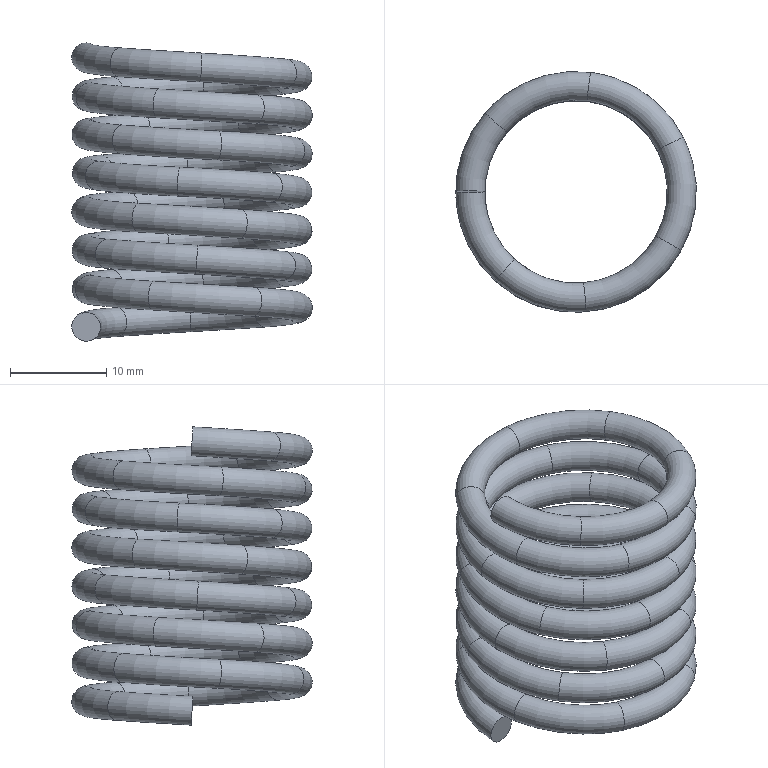Part | NX | features solid 2 | 1 solid | 48 faces | box 25.01 x 25.011 x 30.995 mm | volume 3423 mm3 | torus 46 | plane 2
STEP:
#1=CARTESIAN_POINT('',(-1547.251,422.027,-15.808));
#2=VERTEX_POINT('',#1);
#3=CARTESIAN_POINT('',(-1547.85,422.702,-17.006));
#4=DIRECTION('',(-0.6998,-0.7125,-0.05188));
#5=DIRECTION('',(0.3989,-0.45,0.799));
#6=AXIS2_PLACEMENT_3D('',#3,#4,#5);
#7=CIRCLE('',#6,1.5);
#8=EDGE_CURVE('',#2,#2,#7,.T.);
#9=ORIENTED_EDGE('',*,*,#8,.T.);
#10=EDGE_LOOP('',(#9));
#11=FACE_BOUND('',#10,.T.);
#12=CARTESIAN_POINT('',(-1550.155,414.928,-16.263));
#13=VERTEX_POINT('',#12);
#14=CARTESIAN_POINT('',(-1551.,415.,-17.5));
#15=DIRECTION('',(0.,-0.9983,-0.05778));
#16=DIRECTION('',(0.5635,-0.04773,0.8248));
#17=AXIS2_PLACEMENT_3D('',#14,#15,#16);
#18=CIRCLE('',#17,1.5);
#19=EDGE_CURVE('',#13,#13,#18,.T.);
#20=ORIENTED_EDGE('',*,*,#19,.F.);
#21=EDGE_LOOP('',(#20));
#22=FACE_BOUND('',#21,.T.);
#23=CARTESIAN_POINT('',(-1539.974,414.99,-17.333));
#24=DIRECTION('',(-0.01519,-0.05777,0.9982));
#25=DIRECTION('',(0.,-0.9983,-0.05778));
#26=AXIS2_PLACEMENT_3D('',#23,#24,#25);
#27=TOROIDAL_SURFACE('',#26,11.027,1.5);
#28=ADVANCED_FACE('',(#11,#22),#27,.T.);
#29=CARTESIAN_POINT('',(-1540.254,425.044,-15.355));
#30=VERTEX_POINT('',#29);
#31=CARTESIAN_POINT('',(-1540.206,425.998,-16.512));
#32=DIRECTION('',(-0.9981,-0.01974,-0.05793));
#33=DIRECTION('',(-0.03218,-0.6359,0.7711));
#34=AXIS2_PLACEMENT_3D('',#31,#32,#33);
#35=CIRCLE('',#34,1.5);
#36=EDGE_CURVE('',#30,#30,#35,.T.);
#37=ORIENTED_EDGE('',*,*,#36,.T.);
#38=EDGE_LOOP('',(#37));
#39=FACE_BOUND('',#38,.T.);
#40=ORIENTED_EDGE('',*,*,#8,.F.);
#41=EDGE_LOOP('',(#40));
#42=FACE_BOUND('',#41,.T.);
#43=CARTESIAN_POINT('',(-1539.978,414.946,-16.677));
#44=DIRECTION('',(-0.05762,-0.0161,0.9982));
#45=DIRECTION('',(0.9983,0.,0.05762));
#46=AXIS2_PLACEMENT_3D('',#43,#44,#45);
#47=TOROIDAL_SURFACE('',#46,11.056,1.5);
#48=ADVANCED_FACE('',(#39,#42),#47,.T.);
#49=CARTESIAN_POINT('',(-1533.181,422.306,-14.905));
#50=VERTEX_POINT('',#49);
#51=CARTESIAN_POINT('',(-1532.449,422.995,-16.018));
#52=DIRECTION('',(-0.725,0.6868,-0.05181));
#53=DIRECTION('',(-0.4882,-0.4594,0.742));
#54=AXIS2_PLACEMENT_3D('',#51,#52,#53);
#55=CIRCLE('',#54,1.5);
#56=EDGE_CURVE('',#50,#50,#55,.T.);
#57=ORIENTED_EDGE('',*,*,#56,.T.);
#58=EDGE_LOOP('',(#57));
#59=FACE_BOUND('',#58,.T.);
#60=ORIENTED_EDGE('',*,*,#36,.F.);
#61=EDGE_LOOP('',(#60));
#62=FACE_BOUND('',#61,.T.);
#63=CARTESIAN_POINT('',(-1539.998,415.002,-16.347));
#64=DIRECTION('',(-0.05821,0.01386,0.9982));
#65=DIRECTION('',(0.9983,0.,0.05821));
#66=AXIS2_PLACEMENT_3D('',#63,#64,#65);
#67=TOROIDAL_SURFACE('',#66,11.,1.5);
#68=ADVANCED_FACE('',(#59,#62),#67,.T.);
#69=CARTESIAN_POINT('',(-1530.062,415.432,-14.457));
#70=VERTEX_POINT('',#69);
#71=CARTESIAN_POINT('',(-1529.008,415.412,-15.524));
#72=DIRECTION('',(-0.03934,0.9975,-0.05792));
#73=DIRECTION('',(-0.7028,0.01358,0.7112));
#74=AXIS2_PLACEMENT_3D('',#71,#72,#73);
#75=CIRCLE('',#74,1.5);
#76=EDGE_CURVE('',#70,#70,#75,.T.);
#77=ORIENTED_EDGE('',*,*,#76,.T.);
#78=EDGE_LOOP('',(#77));
#79=FACE_BOUND('',#78,.T.);
#80=ORIENTED_EDGE('',*,*,#56,.F.);
#81=EDGE_LOOP('',(#80));
#82=FACE_BOUND('',#81,.T.);
#83=CARTESIAN_POINT('',(-1540.079,414.966,-15.688));
#84=DIRECTION('',(-0.01706,0.05729,0.9982));
#85=DIRECTION('',(0.,-0.9984,0.0573));
#86=AXIS2_PLACEMENT_3D('',#83,#84,#85);
#87=TOROIDAL_SURFACE('',#86,11.081,1.5);
#88=ADVANCED_FACE('',(#79,#82),#87,.T.);
#89=CARTESIAN_POINT('',(-1534.223,406.975,-13.888));
#90=VERTEX_POINT('',#89);
#91=CARTESIAN_POINT('',(-1533.618,406.04,-14.893));
#92=DIRECTION('',(0.8145,0.5782,-0.04816));
#93=DIRECTION('',(-0.4029,0.6233,0.6702));
#94=AXIS2_PLACEMENT_3D('',#91,#92,#93);
#95=CIRCLE('',#94,1.5);
#96=EDGE_CURVE('',#90,#90,#95,.T.);
#97=ORIENTED_EDGE('',*,*,#96,.T.);
#98=EDGE_LOOP('',(#97));
#99=FACE_BOUND('',#98,.T.);
#100=ORIENTED_EDGE('',*,*,#76,.F.);
#101=EDGE_LOOP('',(#100));
#102=FACE_BOUND('',#101,.T.);
#103=CARTESIAN_POINT('',(-1539.997,414.991,-15.308));
#104=DIRECTION('',(0.01738,0.05864,0.9981));
#105=DIRECTION('',(0.,-0.9983,0.05865));
#106=AXIS2_PLACEMENT_3D('',#103,#104,#105);
#107=TOROIDAL_SURFACE('',#106,10.999,1.5);
#108=ADVANCED_FACE('',(#99,#102),#107,.T.);
#109=CARTESIAN_POINT('',(-1543.516,405.833,-13.323));
#110=VERTEX_POINT('',#109);
#111=CARTESIAN_POINT('',(-1543.992,404.765,-14.263));
#112=DIRECTION('',(0.9297,-0.3638,-0.05774));
#113=DIRECTION('',(0.3175,0.7119,0.6264));
#114=AXIS2_PLACEMENT_3D('',#111,#112,#113);
#115=CIRCLE('',#114,1.5);
#116=EDGE_CURVE('',#110,#110,#115,.T.);
#117=ORIENTED_EDGE('',*,*,#116,.T.);
#118=EDGE_LOOP('',(#117));
#119=FACE_BOUND('',#118,.T.);
#120=ORIENTED_EDGE('',*,*,#96,.F.);
#121=EDGE_LOOP('',(#120));
#122=FACE_BOUND('',#121,.T.);
#123=CARTESIAN_POINT('',(-1539.984,415.041,-14.48));
#124=DIRECTION('',(0.06093,-0.002702,0.9981));
#125=DIRECTION('',(0.9981,0.,-0.06093));
#126=AXIS2_PLACEMENT_3D('',#123,#124,#125);
#127=TOROIDAL_SURFACE('',#126,11.033,1.5);
#128=ADVANCED_FACE('',(#119,#122),#127,.T.);
#129=CARTESIAN_POINT('',(-1549.456,412.582,-12.782));
#130=VERTEX_POINT('',#129);
#131=CARTESIAN_POINT('',(-1550.647,412.328,-13.657));
#132=DIRECTION('',(0.243,-0.9688,-0.04909));
#133=DIRECTION('',(0.7946,0.1697,0.583));
#134=AXIS2_PLACEMENT_3D('',#131,#132,#133);
#135=CIRCLE('',#134,1.5);
#136=EDGE_CURVE('',#130,#130,#135,.T.);
#137=ORIENTED_EDGE('',*,*,#136,.T.);
#138=EDGE_LOOP('',(#137));
#139=FACE_BOUND('',#138,.T.);
#140=ORIENTED_EDGE('',*,*,#116,.F.);
#141=EDGE_LOOP('',(#140));
#142=FACE_BOUND('',#141,.T.);
#143=CARTESIAN_POINT('',(-1539.963,415.027,-14.053));
#144=DIRECTION('',(0.04679,-0.03884,0.9981));
#145=DIRECTION('',(0.9989,0.,-0.04683));
#146=AXIS2_PLACEMENT_3D('',#143,#144,#145);
#147=TOROIDAL_SURFACE('',#146,11.027,1.5);
#148=ADVANCED_FACE('',(#139,#142),#147,.T.);
#149=CARTESIAN_POINT('',(-1547.425,421.291,-12.244));
#150=VERTEX_POINT('',#149);
#151=CARTESIAN_POINT('',(-1548.358,422.145,-13.05));
#152=DIRECTION('',(-0.6463,-0.7609,-0.05788));
#153=DIRECTION('',(0.6222,-0.5694,0.5373));
#154=AXIS2_PLACEMENT_3D('',#151,#152,#153);
#155=CIRCLE('',#154,1.5);
#156=EDGE_CURVE('',#150,#150,#155,.T.);
#157=ORIENTED_EDGE('',*,*,#156,.T.);
#158=EDGE_LOOP('',(#157));
#159=FACE_BOUND('',#158,.T.);
#160=ORIENTED_EDGE('',*,*,#136,.F.);
#161=EDGE_LOOP('',(#160));
#162=FACE_BOUND('',#161,.T.);
#163=CARTESIAN_POINT('',(-1539.924,414.997,-13.259));
#164=DIRECTION('',(-0.02304,-0.05635,0.9981));
#165=DIRECTION('',(0.,-0.9984,-0.05637));
#166=AXIS2_PLACEMENT_3D('',#163,#164,#165);
#167=TOROIDAL_SURFACE('',#166,11.057,1.5);
#168=ADVANCED_FACE('',(#159,#162),#167,.T.);
#169=CARTESIAN_POINT('',(-1538.882,424.631,-11.69));
#170=VERTEX_POINT('',#169);
#171=CARTESIAN_POINT('',(-1538.689,425.925,-12.423));
#172=DIRECTION('',(-0.9915,0.1205,-0.04827));
#173=DIRECTION('',(-0.1286,-0.863,0.4886));
#174=AXIS2_PLACEMENT_3D('',#171,#172,#173);
#175=CIRCLE('',#174,1.5);
#176=EDGE_CURVE('',#170,#170,#175,.T.);
#177=ORIENTED_EDGE('',*,*,#176,.T.);
#178=EDGE_LOOP('',(#177));
#179=FACE_BOUND('',#178,.T.);
#180=ORIENTED_EDGE('',*,*,#156,.F.);
#181=EDGE_LOOP('',(#180));
#182=FACE_BOUND('',#181,.T.);
#183=CARTESIAN_POINT('',(-1539.994,415.023,-12.835));
#184=DIRECTION('',(-0.0524,-0.03142,0.9981));
#185=DIRECTION('',(0.9986,0.,0.05243));
#186=AXIS2_PLACEMENT_3D('',#183,#184,#185);
#187=TOROIDAL_SURFACE('',#186,10.987,1.5);
#188=ADVANCED_FACE('',(#179,#182),#187,.T.);
#189=CARTESIAN_POINT('',(-1531.412,419.377,-11.14));
#190=VERTEX_POINT('',#189);
#191=CARTESIAN_POINT('',(-1530.191,419.947,-11.797));
#192=DIRECTION('',(-0.448,0.8921,-0.05774));
#193=DIRECTION('',(-0.8144,-0.3806,0.4381));
#194=AXIS2_PLACEMENT_3D('',#191,#192,#193);
#195=CIRCLE('',#194,1.5);
#196=EDGE_CURVE('',#190,#190,#195,.T.);
#197=ORIENTED_EDGE('',*,*,#196,.T.);
#198=EDGE_LOOP('',(#197));
#199=FACE_BOUND('',#198,.T.);
#200=ORIENTED_EDGE('',*,*,#176,.F.);
#201=EDGE_LOOP('',(#200));
#202=FACE_BOUND('',#201,.T.);
#203=CARTESIAN_POINT('',(-1540.038,414.988,-12.013));
#204=DIRECTION('',(-0.04338,0.04282,0.9981));
#205=DIRECTION('',(0.9991,0.,0.04342));
#206=AXIS2_PLACEMENT_3D('',#203,#204,#205);
#207=TOROIDAL_SURFACE('',#206,11.028,1.5);
#208=ADVANCED_FACE('',(#199,#202),#207,.T.);
#209=CARTESIAN_POINT('',(-1531.72,410.149,-10.583));
#210=VERTEX_POINT('',#209);
#211=CARTESIAN_POINT('',(-1530.541,409.424,-11.162));
#212=DIRECTION('',(0.5065,0.8609,-0.04814));
#213=DIRECTION('',(-0.7856,0.4837,0.3859));
#214=AXIS2_PLACEMENT_3D('',#211,#212,#213);
#215=CIRCLE('',#214,1.5);
#216=EDGE_CURVE('',#210,#210,#215,.T.);
#217=ORIENTED_EDGE('',*,*,#216,.T.);
#218=EDGE_LOOP('',(#217));
#219=FACE_BOUND('',#218,.T.);
#220=ORIENTED_EDGE('',*,*,#196,.F.);
#221=EDGE_LOOP('',(#220));
#222=FACE_BOUND('',#221,.T.);
#223=CARTESIAN_POINT('',(-1540.065,415.003,-11.577));
#224=DIRECTION('',(-0.00806,0.06056,0.9981));
#225=DIRECTION('',(0.,-0.9982,0.06056));
#226=AXIS2_PLACEMENT_3D('',#223,#224,#225);
#227=TOROIDAL_SURFACE('',#226,11.045,1.5);
#228=ADVANCED_FACE('',(#219,#222),#227,.T.);
#229=CARTESIAN_POINT('',(-1539.599,405.424,-10.027));
#230=VERTEX_POINT('',#229);
#231=CARTESIAN_POINT('',(-1539.569,404.009,-10.525));
#232=DIRECTION('',(0.9975,0.04112,-0.05792));
#233=DIRECTION('',(-0.0196,0.9431,0.3319));
#234=AXIS2_PLACEMENT_3D('',#231,#232,#233);
#235=CIRCLE('',#234,1.5);
#236=EDGE_CURVE('',#230,#230,#235,.T.);
#237=ORIENTED_EDGE('',*,*,#236,.T.);
#238=EDGE_LOOP('',(#237));
#239=FACE_BOUND('',#238,.T.);
#240=ORIENTED_EDGE('',*,*,#216,.F.);
#241=EDGE_LOOP('',(#240));
#242=FACE_BOUND('',#241,.T.);
#243=CARTESIAN_POINT('',(-1540.036,415.033,-10.744));
#244=DIRECTION('',(0.05704,0.02226,0.9981));
#245=DIRECTION('',(0.9984,0.,-0.05706));
#246=AXIS2_PLACEMENT_3D('',#243,#244,#245);
#247=TOROIDAL_SURFACE('',#246,11.036,1.5);
#248=ADVANCED_FACE('',(#239,#242),#247,.T.);
#249=CARTESIAN_POINT('',(-1547.65,409.26,-9.49));
#250=VERTEX_POINT('',#249);
#251=CARTESIAN_POINT('',(-1548.817,408.415,-9.908));
#252=DIRECTION('',(0.597,-0.8008,-0.04853));
#253=DIRECTION('',(0.778,0.5631,0.2787));
#254=AXIS2_PLACEMENT_3D('',#251,#252,#253);
#255=CIRCLE('',#254,1.5);
#256=EDGE_CURVE('',#250,#250,#255,.T.);
#257=ORIENTED_EDGE('',*,*,#256,.T.);
#258=EDGE_LOOP('',(#257));
#259=FACE_BOUND('',#258,.T.);
#260=ORIENTED_EDGE('',*,*,#236,.F.);
#261=EDGE_LOOP('',(#260));
#262=FACE_BOUND('',#261,.T.);
#263=CARTESIAN_POINT('',(-1540.01,415.005,-10.314));
#264=DIRECTION('',(0.05865,-0.01676,0.9981));
#265=DIRECTION('',(0.9983,0.,-0.05866));
#266=AXIS2_PLACEMENT_3D('',#263,#264,#265);
#267=TOROIDAL_SURFACE('',#266,11.007,1.5);
#268=ADVANCED_FACE('',(#259,#262),#267,.T.);
#269=CARTESIAN_POINT('',(-1549.026,418.045,-8.955));
#270=VERTEX_POINT('',#269);
#271=CARTESIAN_POINT('',(-1550.402,418.537,-9.291));
#272=DIRECTION('',(-0.3236,-0.9444,-0.05775));
#273=DIRECTION('',(0.9176,-0.3282,0.2244));
#274=AXIS2_PLACEMENT_3D('',#271,#272,#273);
#275=CIRCLE('',#274,1.5);
#276=EDGE_CURVE('',#270,#270,#275,.T.);
#277=ORIENTED_EDGE('',*,*,#276,.T.);
#278=EDGE_LOOP('',(#277));
#279=FACE_BOUND('',#278,.T.);
#280=ORIENTED_EDGE('',*,*,#256,.F.);
#281=EDGE_LOOP('',(#280));
#282=FACE_BOUND('',#281,.T.);
#283=CARTESIAN_POINT('',(-1539.98,414.978,-9.503));
#284=DIRECTION('',(-0.0005035,-0.06086,0.9981));
#285=DIRECTION('',(0.,-0.9981,-0.06086));
#286=AXIS2_PLACEMENT_3D('',#283,#284,#285);
#287=TOROIDAL_SURFACE('',#286,11.015,1.5);
#288=ADVANCED_FACE('',(#279,#282),#287,.T.);
#289=CARTESIAN_POINT('',(-1542.436,424.179,-8.412));
#290=VERTEX_POINT('',#289);
#291=CARTESIAN_POINT('',(-1542.802,425.612,-8.665));
#292=DIRECTION('',(-0.9655,-0.2557,-0.04849));
#293=DIRECTION('',(0.2444,-0.9549,0.1689));
#294=AXIS2_PLACEMENT_3D('',#291,#292,#293);
#295=CIRCLE('',#294,1.5);
#296=EDGE_CURVE('',#290,#290,#295,.T.);
#297=ORIENTED_EDGE('',*,*,#296,.T.);
#298=EDGE_LOOP('',(#297));
#299=FACE_BOUND('',#298,.T.);
#300=ORIENTED_EDGE('',*,*,#276,.F.);
#301=EDGE_LOOP('',(#300));
#302=FACE_BOUND('',#301,.T.);
#303=CARTESIAN_POINT('',(-1539.957,414.944,-9.074));
#304=DIRECTION('',(-0.03735,-0.04823,0.9981));
#305=DIRECTION('',(0.,-0.9988,-0.04827));
#306=AXIS2_PLACEMENT_3D('',#303,#304,#305);
#307=TOROIDAL_SURFACE('',#306,11.048,1.5);
#308=ADVANCED_FACE('',(#299,#302),#307,.T.);
#309=CARTESIAN_POINT('',(-1533.693,422.112,-7.869));
#310=VERTEX_POINT('',#309);
#311=CARTESIAN_POINT('',(-1532.699,423.223,-8.038));
#312=DIRECTION('',(-0.7482,0.6609,-0.05789));
#313=DIRECTION('',(-0.6627,-0.7404,0.1126));
#314=AXIS2_PLACEMENT_3D('',#311,#312,#313);
#315=CIRCLE('',#314,1.5);
#316=EDGE_CURVE('',#310,#310,#315,.T.);
#317=ORIENTED_EDGE('',*,*,#316,.T.);
#318=EDGE_LOOP('',(#317));
#319=FACE_BOUND('',#318,.T.);
#320=ORIENTED_EDGE('',*,*,#296,.F.);
#321=EDGE_LOOP('',(#320));
#322=FACE_BOUND('',#321,.T.);
#323=CARTESIAN_POINT('',(-1539.997,414.941,-8.254));
#324=DIRECTION('',(-0.05637,0.0236,0.9981));
#325=DIRECTION('',(0.9984,0.,0.05639));
#326=AXIS2_PLACEMENT_3D('',#323,#324,#325);
#327=TOROIDAL_SURFACE('',#326,11.041,1.5);
#328=ADVANCED_FACE('',(#319,#322),#327,.T.);
#329=CARTESIAN_POINT('',(-1530.566,413.83,-7.335));
#330=VERTEX_POINT('',#329);
#331=CARTESIAN_POINT('',(-1529.081,413.639,-7.42));
#332=DIRECTION('',(0.1246,0.991,-0.04854));
#333=DIRECTION('',(-0.9902,0.1273,0.05669));
#334=AXIS2_PLACEMENT_3D('',#331,#332,#333);
#335=CIRCLE('',#334,1.5);
#336=EDGE_CURVE('',#330,#330,#335,.T.);
#337=ORIENTED_EDGE('',*,*,#336,.T.);
#338=EDGE_LOOP('',(#337));
#339=FACE_BOUND('',#338,.T.);
#340=ORIENTED_EDGE('',*,*,#316,.F.);
#341=EDGE_LOOP('',(#340));
#342=FACE_BOUND('',#341,.T.);
#343=CARTESIAN_POINT('',(-1539.986,414.991,-7.826));
#344=DIRECTION('',(-0.03063,0.05275,0.9981));
#345=DIRECTION('',(0.,-0.9986,0.05277));
#346=AXIS2_PLACEMENT_3D('',#343,#344,#345);
#347=TOROIDAL_SURFACE('',#346,10.996,1.5);
#348=ADVANCED_FACE('',(#339,#342),#347,.T.);
#349=CARTESIAN_POINT('',(-1535.64,406.574,-6.803));
#350=VERTEX_POINT('',#349);
#351=CARTESIAN_POINT('',(-1534.954,405.24,-6.804));
#352=DIRECTION('',(0.8877,0.4567,-0.05775));
#353=DIRECTION('',(-0.4574,0.8892,0.000754));
#354=AXIS2_PLACEMENT_3D('',#351,#352,#353);
#355=CIRCLE('',#354,1.5);
#356=EDGE_CURVE('',#350,#350,#355,.T.);
#357=ORIENTED_EDGE('',*,*,#356,.T.);
#358=EDGE_LOOP('',(#357));
#359=FACE_BOUND('',#358,.T.);
#360=ORIENTED_EDGE('',*,*,#336,.F.);
#361=EDGE_LOOP('',(#360));
#362=FACE_BOUND('',#361,.T.);
#363=CARTESIAN_POINT('',(-1540.006,415.033,-7.016));
#364=DIRECTION('',(0.04253,0.04355,0.9981));
#365=DIRECTION('',(0.,-0.999,0.04359));
#366=AXIS2_PLACEMENT_3D('',#363,#364,#365);
#367=TOROIDAL_SURFACE('',#366,11.021,1.5);
#368=ADVANCED_FACE('',(#359,#362),#367,.T.);
#369=CARTESIAN_POINT('',(-1544.747,406.793,-6.253));
#370=VERTEX_POINT('',#369);
#371=CARTESIAN_POINT('',(-1545.492,405.494,-6.167));
#372=DIRECTION('',(0.8653,-0.4989,-0.04813));
#373=DIRECTION('',(0.4963,0.8663,-0.05685));
#374=AXIS2_PLACEMENT_3D('',#371,#372,#373);
#375=CIRCLE('',#374,1.5);
#376=EDGE_CURVE('',#370,#370,#375,.T.);
#377=ORIENTED_EDGE('',*,*,#376,.T.);
#378=EDGE_LOOP('',(#377));
#379=FACE_BOUND('',#378,.T.);
#380=ORIENTED_EDGE('',*,*,#356,.F.);
#381=EDGE_LOOP('',(#380));
#382=FACE_BOUND('',#381,.T.);
#383=CARTESIAN_POINT('',(-1539.995,415.067,-6.583));
#384=DIRECTION('',(0.06049,0.008624,0.9981));
#385=DIRECTION('',(0.9982,0.,-0.06049));
#386=AXIS2_PLACEMENT_3D('',#383,#384,#385);
#387=TOROIDAL_SURFACE('',#386,11.047,1.5);
#388=ADVANCED_FACE('',(#379,#382),#387,.T.);
#389=CARTESIAN_POINT('',(-1549.5,414.569,-5.701));
#390=VERTEX_POINT('',#389);
#391=CARTESIAN_POINT('',(-1550.987,414.486,-5.53));
#392=DIRECTION('',(0.04897,-0.9971,-0.05792));
#393=DIRECTION('',(0.9919,0.05536,-0.1143));
#394=AXIS2_PLACEMENT_3D('',#391,#392,#393);
#395=CIRCLE('',#394,1.5);
#396=EDGE_CURVE('',#390,#390,#395,.T.);
#397=ORIENTED_EDGE('',*,*,#396,.T.);
#398=EDGE_LOOP('',(#397));
#399=FACE_BOUND('',#398,.T.);
#400=ORIENTED_EDGE('',*,*,#376,.F.);
#401=EDGE_LOOP('',(#400));
#402=FACE_BOUND('',#401,.T.);
#403=CARTESIAN_POINT('',(-1539.965,415.04,-5.749));
#404=DIRECTION('',(0.02274,-0.05686,0.9981));
#405=DIRECTION('',(0.,-0.9984,-0.05688));
#406=AXIS2_PLACEMENT_3D('',#403,#404,#405);
#407=TOROIDAL_SURFACE('',#406,11.039,1.5);
#408=ADVANCED_FACE('',(#399,#402),#407,.T.);
#409=CARTESIAN_POINT('',(-1545.628,422.685,-5.158));
#410=VERTEX_POINT('',#409);
#411=CARTESIAN_POINT('',(-1546.511,423.87,-4.902));
#412=DIRECTION('',(-0.8061,-0.5899,-0.04823));
#413=DIRECTION('',(0.5885,-0.7902,-0.1709));
#414=AXIS2_PLACEMENT_3D('',#411,#412,#413);
#415=CIRCLE('',#414,1.5);
#416=EDGE_CURVE('',#410,#410,#415,.T.);
#417=ORIENTED_EDGE('',*,*,#416,.T.);
#418=EDGE_LOOP('',(#417));
#419=FACE_BOUND('',#418,.T.);
#420=ORIENTED_EDGE('',*,*,#396,.F.);
#421=EDGE_LOOP('',(#420));
#422=FACE_BOUND('',#421,.T.);
#423=CARTESIAN_POINT('',(-1540.004,415.013,-5.315));
#424=DIRECTION('',(-0.01669,-0.0588,0.9981));
#425=DIRECTION('',(0.,-0.9983,-0.05881));
#426=AXIS2_PLACEMENT_3D('',#423,#424,#425);
#427=TOROIDAL_SURFACE('',#426,10.998,1.5);
#428=ADVANCED_FACE('',(#419,#422),#427,.T.);
#429=CARTESIAN_POINT('',(-1536.696,423.934,-4.615));
#430=VERTEX_POINT('',#429);
#431=CARTESIAN_POINT('',(-1536.207,425.311,-4.276));
#432=DIRECTION('',(-0.9364,0.3462,-0.05774));
#433=DIRECTION('',(-0.3255,-0.918,-0.2265));
#434=AXIS2_PLACEMENT_3D('',#431,#432,#433);
#435=CIRCLE('',#434,1.5);
#436=EDGE_CURVE('',#430,#430,#435,.T.);
#437=ORIENTED_EDGE('',*,*,#436,.T.);
#438=EDGE_LOOP('',(#437));
#439=FACE_BOUND('',#438,.T.);
#440=ORIENTED_EDGE('',*,*,#416,.F.);
#441=EDGE_LOOP('',(#440));
#442=FACE_BOUND('',#441,.T.);
#443=CARTESIAN_POINT('',(-1540.019,414.966,-4.491));
#444=DIRECTION('',(-0.06094,0.001658,0.9981));
#445=DIRECTION('',(0.9981,0.,0.06094));
#446=AXIS2_PLACEMENT_3D('',#443,#444,#445);
#447=TOROIDAL_SURFACE('',#446,11.027,1.5);
#448=ADVANCED_FACE('',(#439,#442),#447,.T.);
#449=CARTESIAN_POINT('',(-1530.749,417.322,-4.079));
#450=VERTEX_POINT('',#449);
#451=CARTESIAN_POINT('',(-1529.359,417.695,-3.658));
#452=DIRECTION('',(-0.2456,0.9682,-0.04876));
#453=DIRECTION('',(-0.9269,-0.2492,-0.2807));
#454=AXIS2_PLACEMENT_3D('',#451,#452,#453);
#455=CIRCLE('',#454,1.5);
#456=EDGE_CURVE('',#450,#450,#455,.T.);
#457=ORIENTED_EDGE('',*,*,#456,.T.);
#458=EDGE_LOOP('',(#457));
#459=FACE_BOUND('',#458,.T.);
#460=ORIENTED_EDGE('',*,*,#436,.F.);
#461=EDGE_LOOP('',(#460));
#462=FACE_BOUND('',#461,.T.);
#463=CARTESIAN_POINT('',(-1540.046,414.964,-4.061));
#464=DIRECTION('',(-0.04741,0.03824,0.9981));
#465=DIRECTION('',(0.9989,0.,0.04745));
#466=AXIS2_PLACEMENT_3D('',#463,#464,#465);
#467=TOROIDAL_SURFACE('',#466,11.038,1.5);
#468=ADVANCED_FACE('',(#459,#462),#467,.T.);
#469=CARTESIAN_POINT('',(-1532.829,408.643,-3.541));
#470=VERTEX_POINT('',#469);
#471=CARTESIAN_POINT('',(-1531.747,407.734,-3.041));
#472=DIRECTION('',(0.6577,0.7511,-0.05789));
#473=DIRECTION('',(-0.7218,0.6063,-0.3337));
#474=AXIS2_PLACEMENT_3D('',#471,#472,#473);
#475=CIRCLE('',#474,1.5);
#476=EDGE_CURVE('',#470,#470,#475,.T.);
#477=ORIENTED_EDGE('',*,*,#476,.T.);
#478=EDGE_LOOP('',(#477));
#479=FACE_BOUND('',#478,.T.);
#480=ORIENTED_EDGE('',*,*,#456,.F.);
#481=EDGE_LOOP('',(#480));
#482=FACE_BOUND('',#481,.T.);
#483=CARTESIAN_POINT('',(-1540.065,415.,-3.253));
#484=DIRECTION('',(0.02361,0.05626,0.9981));
#485=DIRECTION('',(0.,-0.9984,0.05627));
#486=AXIS2_PLACEMENT_3D('',#483,#484,#485);
#487=TOROIDAL_SURFACE('',#486,11.047,1.5);
#488=ADVANCED_FACE('',(#479,#482),#487,.T.);
#489=CARTESIAN_POINT('',(-1541.183,405.452,-3.002));
#490=VERTEX_POINT('',#489);
#491=CARTESIAN_POINT('',(-1541.323,404.076,-2.423));
#492=DIRECTION('',(0.9914,-0.1212,-0.04853));
#493=DIRECTION('',(0.09324,0.9176,-0.3863));
#494=AXIS2_PLACEMENT_3D('',#491,#492,#493);
#495=CIRCLE('',#494,1.5);
#496=EDGE_CURVE('',#490,#490,#495,.T.);
#497=ORIENTED_EDGE('',*,*,#496,.T.);
#498=EDGE_LOOP('',(#497));
#499=FACE_BOUND('',#498,.T.);
#500=ORIENTED_EDGE('',*,*,#476,.F.);
#501=EDGE_LOOP('',(#500));
#502=FACE_BOUND('',#501,.T.);
#503=CARTESIAN_POINT('',(-1540.009,414.984,-2.829));
#504=DIRECTION('',(0.05262,0.03085,0.9981));
#505=DIRECTION('',(0.9986,0.,-0.05265));
#506=AXIS2_PLACEMENT_3D('',#503,#504,#505);
#507=TOROIDAL_SURFACE('',#506,10.995,1.5);
#508=ADVANCED_FACE('',(#499,#502),#507,.T.);
#509=CARTESIAN_POINT('',(-1548.565,410.581,-2.461));
#510=VERTEX_POINT('',#509);
#511=CARTESIAN_POINT('',(-1549.746,409.927,-1.805));
#512=DIRECTION('',(0.4591,-0.8865,-0.05775));
#513=DIRECTION('',(0.7867,0.4359,-0.4371));
#514=AXIS2_PLACEMENT_3D('',#511,#512,#513);
#515=CIRCLE('',#514,1.5);
#516=EDGE_CURVE('',#510,#510,#515,.T.);
#517=ORIENTED_EDGE('',*,*,#516,.T.);
#518=EDGE_LOOP('',(#517));
#519=FACE_BOUND('',#518,.T.);
#520=ORIENTED_EDGE('',*,*,#496,.F.);
#521=EDGE_LOOP('',(#520));
#522=FACE_BOUND('',#521,.T.);
#523=CARTESIAN_POINT('',(-1539.967,415.005,-2.018));
#524=DIRECTION('',(0.04367,-0.0424,0.9981));
#525=DIRECTION('',(0.999,0.,-0.04371));
#526=AXIS2_PLACEMENT_3D('',#523,#524,#525);
#527=TOROIDAL_SURFACE('',#526,11.021,1.5);
#528=ADVANCED_FACE('',(#519,#522),#527,.T.);
#529=CARTESIAN_POINT('',(-1548.364,419.852,-1.901));
#530=VERTEX_POINT('',#529);
#531=CARTESIAN_POINT('',(-1549.517,420.472,-1.169));
#532=DIRECTION('',(-0.4971,-0.8663,-0.04812));
#533=DIRECTION('',(0.7683,-0.4137,-0.4885));
#534=AXIS2_PLACEMENT_3D('',#531,#532,#533);
#535=CIRCLE('',#534,1.5);
#536=EDGE_CURVE('',#530,#530,#535,.T.);
#537=ORIENTED_EDGE('',*,*,#536,.T.);
#538=EDGE_LOOP('',(#537));
#539=FACE_BOUND('',#538,.T.);
#540=ORIENTED_EDGE('',*,*,#516,.F.);
#541=EDGE_LOOP('',(#540));
#542=FACE_BOUND('',#541,.T.);
#543=CARTESIAN_POINT('',(-1539.932,414.995,-1.585));
#544=DIRECTION('',(0.008774,-0.06048,0.9981));
#545=DIRECTION('',(0.,-0.9982,-0.06048));
#546=AXIS2_PLACEMENT_3D('',#543,#544,#545);
#547=TOROIDAL_SURFACE('',#546,11.047,1.5);
#548=ADVANCED_FACE('',(#539,#542),#547,.T.);
#549=CARTESIAN_POINT('',(-1540.417,424.727,-1.337));
#550=VERTEX_POINT('',#549);
#551=CARTESIAN_POINT('',(-1540.528,425.987,-0.5306));
#552=DIRECTION('',(-0.9971,-0.0503,-0.05792));
#553=DIRECTION('',(0.07361,-0.8399,-0.5378));
#554=AXIS2_PLACEMENT_3D('',#551,#552,#553);
#555=CIRCLE('',#554,1.5);
#556=EDGE_CURVE('',#550,#550,#555,.T.);
#557=ORIENTED_EDGE('',*,*,#556,.T.);
#558=EDGE_LOOP('',(#557));
#559=FACE_BOUND('',#558,.T.);
#560=ORIENTED_EDGE('',*,*,#536,.F.);
#561=EDGE_LOOP('',(#560));
#562=FACE_BOUND('',#561,.T.);
#563=CARTESIAN_POINT('',(-1539.959,414.964,-0.7504));
#564=DIRECTION('',(-0.05683,-0.02283,0.9981));
#565=DIRECTION('',(0.9984,0.,0.05685));
#566=AXIS2_PLACEMENT_3D('',#563,#564,#565);
#567=TOROIDAL_SURFACE('',#566,11.039,1.5);
#568=ADVANCED_FACE('',(#559,#562),#567,.T.);
#569=CARTESIAN_POINT('',(-1532.089,420.763,-0.7804));
#570=VERTEX_POINT('',#569);
#571=CARTESIAN_POINT('',(-1531.133,421.516,0.09751));
#572=DIRECTION('',(-0.5903,0.8057,-0.04822));
#573=DIRECTION('',(-0.637,-0.5017,-0.5853));
#574=AXIS2_PLACEMENT_3D('',#571,#572,#573);
#575=CIRCLE('',#574,1.5);
#576=EDGE_CURVE('',#570,#570,#575,.T.);
#577=ORIENTED_EDGE('',*,*,#576,.T.);
#578=EDGE_LOOP('',(#577));
#579=FACE_BOUND('',#578,.T.);
#580=ORIENTED_EDGE('',*,*,#556,.F.);
#581=EDGE_LOOP('',(#580));
#582=FACE_BOUND('',#581,.T.);
#583=CARTESIAN_POINT('',(-1539.986,415.005,-0.3157));
#584=DIRECTION('',(-0.05882,0.01663,0.9981));
#585=DIRECTION('',(0.9983,0.,0.05883));
#586=AXIS2_PLACEMENT_3D('',#583,#584,#585);
#587=TOROIDAL_SURFACE('',#586,10.997,1.5);
#588=ADVANCED_FACE('',(#579,#582),#587,.T.);
#589=CARTESIAN_POINT('',(-1530.8,411.558,-0.2205));
#590=VERTEX_POINT('',#589);
#591=CARTESIAN_POINT('',(-1529.69,411.206,0.7246));
#592=DIRECTION('',(0.3464,0.9363,-0.05774));
#593=DIRECTION('',(-0.7401,0.2349,-0.6301));
#594=AXIS2_PLACEMENT_3D('',#591,#592,#593);
#595=CIRCLE('',#594,1.5);
#596=EDGE_CURVE('',#590,#590,#595,.T.);
#597=ORIENTED_EDGE('',*,*,#596,.T.);
#598=EDGE_LOOP('',(#597));
#599=FACE_BOUND('',#598,.T.);
#600=ORIENTED_EDGE('',*,*,#576,.F.);
#601=EDGE_LOOP('',(#600));
#602=FACE_BOUND('',#601,.T.);
#603=CARTESIAN_POINT('',(-1540.034,415.019,0.5089));
#604=DIRECTION('',(0.001655,0.06094,0.9981));
#605=DIRECTION('',(0.,-0.9981,0.06094));
#606=AXIS2_PLACEMENT_3D('',#603,#604,#605);
#607=TOROIDAL_SURFACE('',#606,11.028,1.5);
#608=ADVANCED_FACE('',(#599,#602),#607,.T.);
#609=CARTESIAN_POINT('',(-1537.634,405.419,0.333));
#610=VERTEX_POINT('',#609);
#611=CARTESIAN_POINT('',(-1537.314,404.356,1.342));
#612=DIRECTION('',(0.9684,0.2447,-0.04874));
#613=DIRECTION('',(-0.2129,0.7085,-0.6728));
#614=AXIS2_PLACEMENT_3D('',#611,#612,#613);
#615=CIRCLE('',#614,1.5);
#616=EDGE_CURVE('',#610,#610,#615,.T.);
#617=ORIENTED_EDGE('',*,*,#616,.T.);
#618=EDGE_LOOP('',(#617));
#619=FACE_BOUND('',#618,.T.);
#620=ORIENTED_EDGE('',*,*,#596,.F.);
#621=EDGE_LOOP('',(#620));
#622=FACE_BOUND('',#621,.T.);
#623=CARTESIAN_POINT('',(-1540.036,415.046,0.9388));
#624=DIRECTION('',(0.03826,0.0474,0.9981));
#625=DIRECTION('',(0.,-0.9989,0.04744));
#626=AXIS2_PLACEMENT_3D('',#623,#624,#625);
#627=TOROIDAL_SURFACE('',#626,11.038,1.5);
#628=ADVANCED_FACE('',(#619,#622),#627,.T.);
#629=CARTESIAN_POINT('',(-1546.633,407.588,0.8914));
#630=VERTEX_POINT('',#629);
#631=CARTESIAN_POINT('',(-1547.28,406.758,1.961));
#632=DIRECTION('',(0.75,-0.6589,-0.05789));
#633=DIRECTION('',(0.4311,0.5533,-0.7127));
#634=AXIS2_PLACEMENT_3D('',#631,#632,#633);
#635=CIRCLE('',#634,1.5);
#636=EDGE_CURVE('',#630,#630,#635,.T.);
#637=ORIENTED_EDGE('',*,*,#636,.T.);
#638=EDGE_LOOP('',(#637));
#639=FACE_BOUND('',#638,.T.);
#640=ORIENTED_EDGE('',*,*,#616,.F.);
#641=EDGE_LOOP('',(#640));
#642=FACE_BOUND('',#641,.T.);
#643=CARTESIAN_POINT('',(-1540.,415.064,1.748));
#644=DIRECTION('',(0.05623,-0.02369,0.9981));
#645=DIRECTION('',(0.9984,0.,-0.05624));
#646=AXIS2_PLACEMENT_3D('',#643,#644,#645);
#647=TOROIDAL_SURFACE('',#646,11.046,1.5);
#648=ADVANCED_FACE('',(#639,#642),#647,.T.);
#649=CARTESIAN_POINT('',(-1549.933,416.28,1.452));
#650=VERTEX_POINT('',#649);
#651=CARTESIAN_POINT('',(-1550.921,416.348,2.579));
#652=DIRECTION('',(-0.1235,-0.9912,-0.04852));
#653=DIRECTION('',(0.6584,-0.04525,-0.7513));
#654=AXIS2_PLACEMENT_3D('',#651,#652,#653);
#655=CIRCLE('',#654,1.5);
#656=EDGE_CURVE('',#650,#650,#655,.T.);
#657=ORIENTED_EDGE('',*,*,#656,.T.);
#658=EDGE_LOOP('',(#657));
#659=FACE_BOUND('',#658,.T.);
#660=ORIENTED_EDGE('',*,*,#636,.F.);
#661=EDGE_LOOP('',(#660));
#662=FACE_BOUND('',#661,.T.);
#663=CARTESIAN_POINT('',(-1540.015,415.009,2.172));
#664=DIRECTION('',(0.03075,-0.05269,0.9981));
#665=DIRECTION('',(0.,-0.9986,-0.05271));
#666=AXIS2_PLACEMENT_3D('',#663,#664,#665);
#667=TOROIDAL_SURFACE('',#666,10.995,1.5);
#668=ADVANCED_FACE('',(#659,#662),#667,.T.);
#669=CARTESIAN_POINT('',(-1544.56,423.971,2.016));
#670=VERTEX_POINT('',#669);
#671=CARTESIAN_POINT('',(-1545.043,424.761,3.196));
#672=DIRECTION('',(-0.8879,-0.4565,-0.05775));
#673=DIRECTION('',(0.322,-0.5267,-0.7867));
#674=AXIS2_PLACEMENT_3D('',#671,#672,#673);
#675=CIRCLE('',#674,1.5);
#676=EDGE_CURVE('',#670,#670,#675,.T.);
#677=ORIENTED_EDGE('',*,*,#676,.T.);
#678=EDGE_LOOP('',(#677));
#679=FACE_BOUND('',#678,.T.);
#680=ORIENTED_EDGE('',*,*,#656,.F.);
#681=EDGE_LOOP('',(#680));
#682=FACE_BOUND('',#681,.T.);
#683=CARTESIAN_POINT('',(-1539.994,414.966,2.984));
#684=DIRECTION('',(-0.04252,-0.04356,0.9981));
#685=DIRECTION('',(0.,-0.999,-0.0436));
#686=AXIS2_PLACEMENT_3D('',#683,#684,#685);
#687=TOROIDAL_SURFACE('',#686,11.022,1.5);
#688=ADVANCED_FACE('',(#679,#682),#687,.T.);
#689=CARTESIAN_POINT('',(-1534.868,423.728,2.602));
#690=VERTEX_POINT('',#689);
#691=CARTESIAN_POINT('',(-1534.491,424.497,3.834));
#692=DIRECTION('',(-0.8645,0.5004,-0.0481));
#693=DIRECTION('',(-0.2509,-0.5124,-0.8213));
#694=AXIS2_PLACEMENT_3D('',#691,#692,#693);
#695=CIRCLE('',#694,1.5);
#696=EDGE_CURVE('',#690,#690,#695,.T.);
#697=ORIENTED_EDGE('',*,*,#696,.T.);
#698=EDGE_LOOP('',(#697));
#699=FACE_BOUND('',#698,.T.);
#700=ORIENTED_EDGE('',*,*,#676,.F.);
#701=EDGE_LOOP('',(#700));
#702=FACE_BOUND('',#701,.T.);
#703=CARTESIAN_POINT('',(-1540.004,414.932,3.417));
#704=DIRECTION('',(-0.06051,-0.008586,0.9981));
#705=DIRECTION('',(0.9982,0.,0.06051));
#706=AXIS2_PLACEMENT_3D('',#703,#704,#705);
#707=TOROIDAL_SURFACE('',#706,11.047,1.5);
#708=ADVANCED_FACE('',(#699,#702),#707,.T.);
#709=CARTESIAN_POINT('',(-1529.788,415.368,3.194));
#710=VERTEX_POINT('',#709);
#711=CARTESIAN_POINT('',(-1529.011,415.478,4.472));
#712=DIRECTION('',(-0.04561,0.9973,-0.05792));
#713=DIRECTION('',(-0.5178,-0.07319,-0.8524));
#714=AXIS2_PLACEMENT_3D('',#711,#712,#713);
#715=CIRCLE('',#714,1.5);
#716=EDGE_CURVE('',#710,#710,#715,.T.);
#717=ORIENTED_EDGE('',*,*,#716,.T.);
#718=EDGE_LOOP('',(#717));
#719=FACE_BOUND('',#718,.T.);
#720=ORIENTED_EDGE('',*,*,#696,.F.);
#721=EDGE_LOOP('',(#720));
#722=FACE_BOUND('',#721,.T.);
#723=CARTESIAN_POINT('',(-1540.034,414.961,4.252));
#724=DIRECTION('',(-0.02258,0.05694,0.9981));
#725=DIRECTION('',(0.,-0.9984,0.05695));
#726=AXIS2_PLACEMENT_3D('',#723,#724,#725);
#727=TOROIDAL_SURFACE('',#726,11.037,1.5);
#728=ADVANCED_FACE('',(#719,#722),#727,.T.);
#729=CARTESIAN_POINT('',(-1533.874,406.722,3.77));
#730=VERTEX_POINT('',#729);
#731=CARTESIAN_POINT('',(-1533.399,406.194,5.091));
#732=DIRECTION('',(0.7998,0.5983,-0.04847));
#733=DIRECTION('',(-0.3168,0.3521,-0.8807));
#734=AXIS2_PLACEMENT_3D('',#731,#732,#733);
#735=CIRCLE('',#734,1.5);
#736=EDGE_CURVE('',#730,#730,#735,.T.);
#737=ORIENTED_EDGE('',*,*,#736,.T.);
#738=EDGE_LOOP('',(#737));
#739=FACE_BOUND('',#738,.T.);
#740=ORIENTED_EDGE('',*,*,#716,.F.);
#741=EDGE_LOOP('',(#740));
#742=FACE_BOUND('',#741,.T.);
#743=CARTESIAN_POINT('',(-1540.002,414.988,4.683));
#744=DIRECTION('',(0.01656,0.05873,0.9981));
#745=DIRECTION('',(0.,-0.9983,0.05874));
#746=AXIS2_PLACEMENT_3D('',#743,#744,#745);
#747=TOROIDAL_SURFACE('',#746,11.004,1.5);
#748=ADVANCED_FACE('',(#739,#742),#747,.T.);
#749=CARTESIAN_POINT('',(-1543.415,405.224,4.351));
#750=VERTEX_POINT('',#749);
#751=CARTESIAN_POINT('',(-1543.546,404.601,5.709));
#752=DIRECTION('',(0.9441,-0.3245,-0.05775));
#753=DIRECTION('',(0.08744,0.4156,-0.9054));
#754=AXIS2_PLACEMENT_3D('',#751,#752,#753);
#755=CIRCLE('',#754,1.5);
#756=EDGE_CURVE('',#750,#750,#755,.T.);
#757=ORIENTED_EDGE('',*,*,#756,.T.);
#758=EDGE_LOOP('',(#757));
#759=FACE_BOUND('',#758,.T.);
#760=ORIENTED_EDGE('',*,*,#736,.F.);
#761=EDGE_LOOP('',(#760));
#762=FACE_BOUND('',#761,.T.);
#763=CARTESIAN_POINT('',(-1539.978,415.022,5.497));
#764=DIRECTION('',(0.06088,-0.0005112,0.9981));
#765=DIRECTION('',(0.9981,0.,-0.06088));
#766=AXIS2_PLACEMENT_3D('',#763,#764,#765);
#767=TOROIDAL_SURFACE('',#766,11.017,1.5);
#768=ADVANCED_FACE('',(#759,#762),#767,.T.);
#769=CARTESIAN_POINT('',(-1550.081,412.362,4.94));
#770=VERTEX_POINT('',#769);
#771=CARTESIAN_POINT('',(-1550.599,412.153,6.332));
#772=DIRECTION('',(0.2596,-0.9645,-0.0486));
#773=DIRECTION('',(0.3451,0.1397,-0.9281));
#774=AXIS2_PLACEMENT_3D('',#771,#772,#773);
#775=CIRCLE('',#774,1.5);
#776=EDGE_CURVE('',#770,#770,#775,.T.);
#777=ORIENTED_EDGE('',*,*,#776,.T.);
#778=EDGE_LOOP('',(#777));
#779=FACE_BOUND('',#778,.T.);
#780=ORIENTED_EDGE('',*,*,#756,.F.);
#781=EDGE_LOOP('',(#780));
#782=FACE_BOUND('',#781,.T.);
#783=CARTESIAN_POINT('',(-1539.945,415.041,5.926));
#784=DIRECTION('',(0.04823,-0.03731,0.9981));
#785=DIRECTION('',(0.9988,0.,-0.04826));
#786=AXIS2_PLACEMENT_3D('',#783,#784,#785);
#787=TOROIDAL_SURFACE('',#786,11.046,1.5);
#788=ADVANCED_FACE('',(#779,#782),#787,.T.);
#789=CARTESIAN_POINT('',(-1547.877,421.976,5.536));
#790=VERTEX_POINT('',#789);
#791=CARTESIAN_POINT('',(-1548.29,422.224,6.956));
#792=DIRECTION('',(-0.6537,-0.7545,-0.05788));
#793=DIRECTION('',(0.2751,-0.1657,-0.947));
#794=AXIS2_PLACEMENT_3D('',#791,#792,#793);
#795=CIRCLE('',#794,1.5);
#796=EDGE_CURVE('',#790,#790,#795,.T.);
#797=ORIENTED_EDGE('',*,*,#796,.T.);
#798=EDGE_LOOP('',(#797));
#799=FACE_BOUND('',#798,.T.);
#800=ORIENTED_EDGE('',*,*,#776,.F.);
#801=EDGE_LOOP('',(#800));
#802=FACE_BOUND('',#801,.T.);
#803=CARTESIAN_POINT('',(-1539.936,415.003,6.741));
#804=DIRECTION('',(-0.02314,-0.05652,0.9981));
#805=DIRECTION('',(0.,-0.9984,-0.05654));
#806=AXIS2_PLACEMENT_3D('',#803,#804,#805);
#807=TOROIDAL_SURFACE('',#806,11.045,1.5);
#808=ADVANCED_FACE('',(#799,#802),#807,.T.);
#809=CARTESIAN_POINT('',(-1538.613,425.519,6.134));
#810=VERTEX_POINT('',#809);
#811=CARTESIAN_POINT('',(-1538.633,425.918,7.58));
#812=DIRECTION('',(-0.9909,0.1255,-0.04836));
#813=DIRECTION('',(0.01337,-0.2658,-0.9639));
#814=AXIS2_PLACEMENT_3D('',#811,#812,#813);
#815=CIRCLE('',#814,1.5);
#816=EDGE_CURVE('',#810,#810,#815,.T.);
#817=ORIENTED_EDGE('',*,*,#816,.T.);
#818=EDGE_LOOP('',(#817));
#819=FACE_BOUND('',#818,.T.);
#820=ORIENTED_EDGE('',*,*,#796,.F.);
#821=EDGE_LOOP('',(#820));
#822=FACE_BOUND('',#821,.T.);
#823=CARTESIAN_POINT('',(-1539.993,415.019,7.17));
#824=DIRECTION('',(-0.05263,-0.03097,0.9981));
#825=DIRECTION('',(0.9986,0.,0.05266));
#826=AXIS2_PLACEMENT_3D('',#823,#824,#825);
#827=TOROIDAL_SURFACE('',#826,10.991,1.5);
#828=ADVANCED_FACE('',(#819,#822),#827,.T.);
#829=CARTESIAN_POINT('',(-1530.426,419.725,6.738));
#830=VERTEX_POINT('',#829);
#831=CARTESIAN_POINT('',(-1530.187,419.94,8.203));
#832=DIRECTION('',(-0.4474,0.8925,-0.05774));
#833=DIRECTION('',(-0.1597,-0.1433,-0.9767));
#834=AXIS2_PLACEMENT_3D('',#831,#832,#833);
#835=CIRCLE('',#834,1.5);
#836=EDGE_CURVE('',#830,#830,#835,.T.);
#837=ORIENTED_EDGE('',*,*,#836,.T.);
#838=EDGE_LOOP('',(#837));
#839=FACE_BOUND('',#838,.T.);
#840=ORIENTED_EDGE('',*,*,#816,.F.);
#841=EDGE_LOOP('',(#840));
#842=FACE_BOUND('',#841,.T.);
#843=CARTESIAN_POINT('',(-1540.037,414.989,7.989));
#844=DIRECTION('',(-0.04328,0.04289,0.9981));
#845=DIRECTION('',(0.9991,0.,0.04332));
#846=AXIS2_PLACEMENT_3D('',#843,#844,#845);
#847=TOROIDAL_SURFACE('',#846,11.027,1.5);
#848=ADVANCED_FACE('',(#839,#842),#847,.T.);
#849=CARTESIAN_POINT('',(-1530.671,409.661,7.345));
#850=VERTEX_POINT('',#849);
#851=CARTESIAN_POINT('',(-1530.438,409.612,8.826));
#852=DIRECTION('',(0.4902,0.8703,-0.04858));
#853=DIRECTION('',(-0.1555,0.03245,-0.9873));
#854=AXIS2_PLACEMENT_3D('',#851,#852,#853);
#855=CIRCLE('',#854,1.5);
#856=EDGE_CURVE('',#850,#850,#855,.T.);
#857=ORIENTED_EDGE('',*,*,#856,.T.);
#858=EDGE_LOOP('',(#857));
#859=FACE_BOUND('',#858,.T.);
#860=ORIENTED_EDGE('',*,*,#836,.F.);
#861=EDGE_LOOP('',(#860));
#862=FACE_BOUND('',#861,.T.);
#863=CARTESIAN_POINT('',(-1540.056,415.007,8.419));
#864=DIRECTION('',(-0.008323,0.06041,0.9981));
#865=DIRECTION('',(0.,-0.9982,0.06041));
#866=AXIS2_PLACEMENT_3D('',#863,#864,#865);
#867=TOROIDAL_SURFACE('',#866,11.035,1.5);
#868=ADVANCED_FACE('',(#859,#862),#867,.T.);
#869=CARTESIAN_POINT('',(-1539.237,404.171,7.959));
#870=VERTEX_POINT('',#869);
#871=CARTESIAN_POINT('',(-1539.139,404.035,9.45));
#872=DIRECTION('',(0.995,0.08159,-0.05791));
#873=DIRECTION('',(-0.06524,0.09028,-0.9938));
#874=AXIS2_PLACEMENT_3D('',#871,#872,#873);
#875=CIRCLE('',#874,1.5);
#876=EDGE_CURVE('',#870,#870,#875,.T.);
#877=ORIENTED_EDGE('',*,*,#876,.T.);
#878=EDGE_LOOP('',(#877));
#879=FACE_BOUND('',#878,.T.);
#880=ORIENTED_EDGE('',*,*,#856,.F.);
#881=EDGE_LOOP('',(#880));
#882=FACE_BOUND('',#881,.T.);
#883=CARTESIAN_POINT('',(-1540.055,415.052,9.235));
#884=DIRECTION('',(0.05611,0.02411,0.9981));
#885=DIRECTION('',(0.9984,0.,-0.05613));
#886=AXIS2_PLACEMENT_3D('',#883,#884,#885);
#887=TOROIDAL_SURFACE('',#886,11.057,1.5);
#888=ADVANCED_FACE('',(#879,#882),#887,.T.);
#889=CARTESIAN_POINT('',(-1547.476,407.019,8.479));
#890=VERTEX_POINT('',#889);
#891=CARTESIAN_POINT('',(-1547.468,406.914,9.975));
#892=DIRECTION('',(0.7326,-0.6788,-0.05098));
#893=DIRECTION('',(-0.005043,0.06948,-0.9976));
#894=AXIS2_PLACEMENT_3D('',#891,#892,#893);
#895=CIRCLE('',#894,1.5);
#896=EDGE_CURVE('',#890,#890,#895,.T.);
#897=ORIENTED_EDGE('',*,*,#896,.T.);
#898=EDGE_LOOP('',(#897));
#899=FACE_BOUND('',#898,.T.);
#900=ORIENTED_EDGE('',*,*,#876,.F.);
#901=EDGE_LOOP('',(#900));
#902=FACE_BOUND('',#901,.T.);
#903=CARTESIAN_POINT('',(-1540.026,414.973,9.626));
#904=DIRECTION('',(0.05902,-0.01127,0.9982));
#905=DIRECTION('',(0.9983,0.,-0.05902));
#906=AXIS2_PLACEMENT_3D('',#903,#904,#905);
#907=TOROIDAL_SURFACE('',#906,10.975,1.5);
#908=ADVANCED_FACE('',(#899,#902),#907,.T.);
#909=ORIENTED_EDGE('',*,*,#19,.T.);
#910=EDGE_LOOP('',(#909));
#911=FACE_BOUND('',#910,.T.);
#912=CARTESIAN_POINT('',(-1551.,415.,-17.5));
#913=DIRECTION('',(0.,-0.9983,-0.05778));
#914=DIRECTION('',(0.5635,-0.04773,0.8248));
#915=AXIS2_PLACEMENT_3D('',#912,#913,#914);
#916=PLANE('',#915);
#917=ADVANCED_FACE('',(#911),#916,.T.);
#918=ORIENTED_EDGE('',*,*,#896,.F.);
#919=EDGE_LOOP('',(#918));
#920=FACE_BOUND('',#919,.T.);
#921=CARTESIAN_POINT('',(-1551.,415.087,9.003));
#922=VERTEX_POINT('',#921);
#923=CARTESIAN_POINT('',(-1551.,415.,10.5));
#924=DIRECTION('',(0.,-0.9983,-0.05793));
#925=DIRECTION('',(0.,0.05793,-0.9983));
#926=AXIS2_PLACEMENT_3D('',#923,#924,#925);
#927=CIRCLE('',#926,1.5);
#928=EDGE_CURVE('',#922,#922,#927,.T.);
#929=ORIENTED_EDGE('',*,*,#928,.T.);
#930=EDGE_LOOP('',(#929));
#931=FACE_BOUND('',#930,.T.);
#932=CARTESIAN_POINT('',(-1539.943,415.01,10.326));
#933=DIRECTION('',(-0.01579,0.05792,-0.9982));
#934=DIRECTION('',(0.,0.9983,0.05793));
#935=AXIS2_PLACEMENT_3D('',#932,#933,#934);
#936=TOROIDAL_SURFACE('',#935,11.059,1.5);
#937=ADVANCED_FACE('',(#920,#931),#936,.T.);
#938=ORIENTED_EDGE('',*,*,#928,.F.);
#939=EDGE_LOOP('',(#938));
#940=FACE_BOUND('',#939,.T.);
#941=CARTESIAN_POINT('',(-1551.,415.,10.5));
#942=DIRECTION('',(0.,-0.9983,-0.05793));
#943=DIRECTION('',(0.,0.05793,-0.9983));
#944=AXIS2_PLACEMENT_3D('',#941,#942,#943);
#945=PLANE('',#944);
#946=ADVANCED_FACE('',(#940),#945,.F.);
#947=CLOSED_SHELL('',(#28,#48,#68,#88,#108,#128,#148,#168,#188,#208,#228,#248,#268,#288,#308,#328,#348,#368,#388,#408,#428,#448,#468,#488,#508,#528,#548,#568,#588,#608,#628,#648,#668,#688,#708,#728,#748,#768,#788,#808,#828,#848,#868,#888,#908,#917,#937,#946));
#948=MANIFOLD_SOLID_BREP('',#947);
#949=(LENGTH_UNIT()NAMED_UNIT(*)SI_UNIT(.MILLI.,.METRE.));
#950=UNCERTAINTY_MEASURE_WITH_UNIT(LENGTH_MEASURE(0.00001),#949,'','');
#951=(NAMED_UNIT(*)PLANE_ANGLE_UNIT()SI_UNIT($,.RADIAN.));
#952=(NAMED_UNIT(*)SI_UNIT($,.STERADIAN.)SOLID_ANGLE_UNIT());
#953=(GEOMETRIC_REPRESENTATION_CONTEXT(3)GLOBAL_UNCERTAINTY_ASSIGNED_CONTEXT((#950))GLOBAL_UNIT_ASSIGNED_CONTEXT((#949,#951,#952))REPRESENTATION_CONTEXT('',''));
#954=ADVANCED_BREP_SHAPE_REPRESENTATION('',(#948),#953);